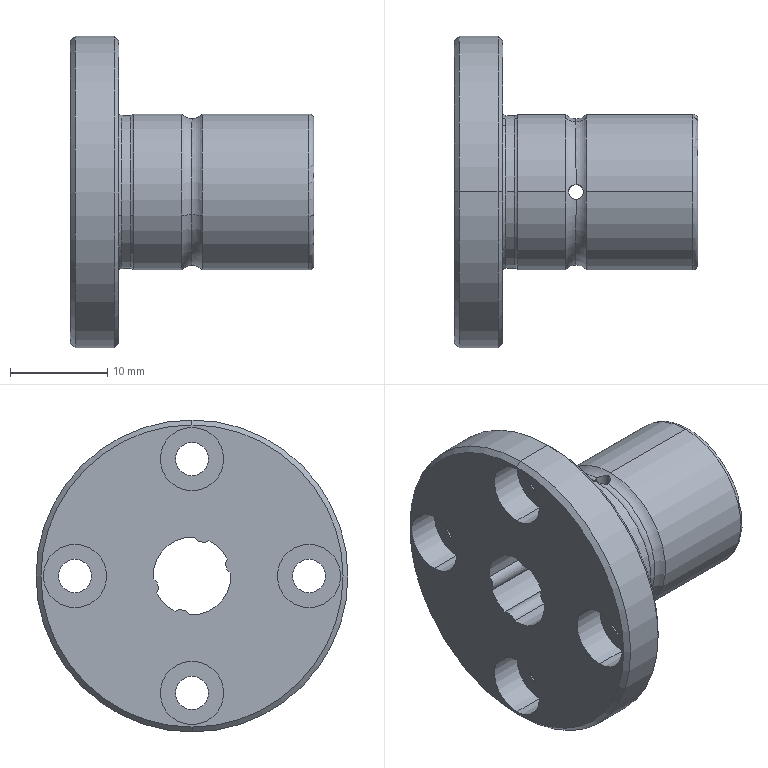Part | SolidWorks | features BaseBody 1 | 1 solid | 57 faces | box 25 x 32 x 32 mm | volume 6244 mm3 | cylinder 36 | torus 10 | plane 7 | cone 4 | commonest cylinder face diameters 3.4 x8 6.5 x8 1.5 x4 2.08 x4 8 x4 16 x4